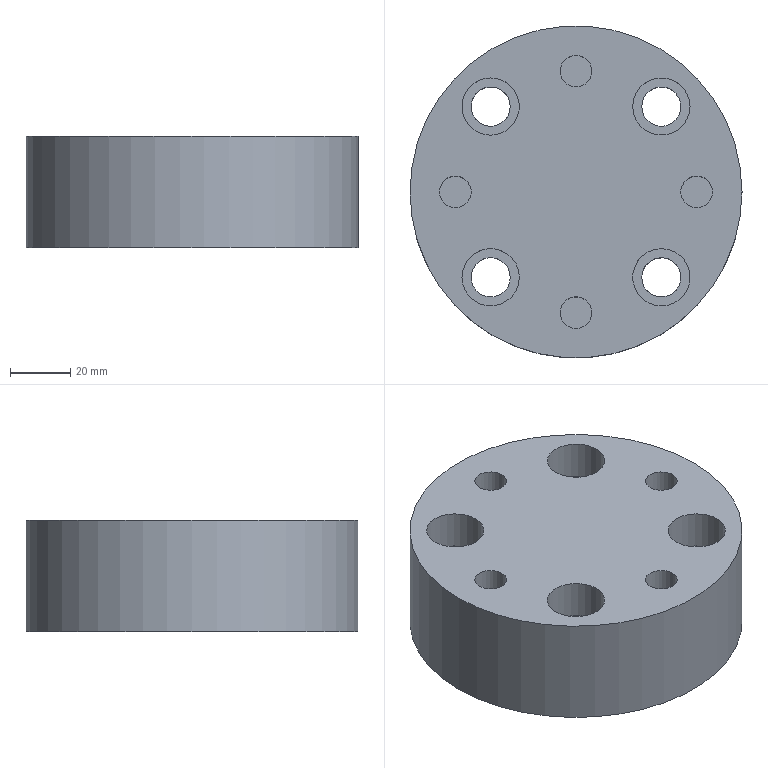CAM job | NX | 3-axis milling, drilling | part box 110 x 110 x 37 mm | stock box 110 x 110 x 37 mm
Tools:
number,name,description,diameter,corner_radius,flute_length,length,flutes
1,ZXZ,Milling Tool-5 Parameters,6.0,0.0,50.0,75.0,2
2,10.5ZT,Drilling Tool,10.5,0.0,35.0,50.0,2
3,13.0ZT,Drilling Tool,13.0,0.0,35.0,50.0,2
10,D10,Milling Tool-5 Parameters,10.0,0.0,50.0,75.0,2
7,D6A45,Milling Tool-5 Parameters,6.0,0.0,50.0,75.0,2
Operations:
program,operation,operation_type,tool,method,geometry_group,spindle_rpm,surface_speed,feed_per_tooth,feed_cut,feed_plunge,cut_length_mm,path_length_mm,cut_time_min,machine_time_min
1,DRILLING,Operation,ZXZ,METHOD,A,3500.0,65.0,0.0357,250.0,0.0,32.0,360.329,0.128,0.1608
1,DRILLING_COPY,Operation,10.5ZT,METHOD,A,1200.0,39.0,0.0625,150.0,0.0,124.618,488.18,0.8308,0.8671
1,DRILLING_COPY_COPY,Operation,13.0ZT,METHOD,A,500.0,20.0,0.15,150.0,0.0,177.622,594.189,1.184,1.226
1,HOLE_MILLING,CylinderMilling,D10,METHOD,A,3000.0,94.0,0.3667,2200.0,100.0,7109.92,7569.626,3.232,3.278
1,PLANAR_MILL,PlanarMilling,D6A45,METHOD,A,7500.0,141.0,0.0833,1250.0,100.0,405.444,1063.216,0.3244,0.3901